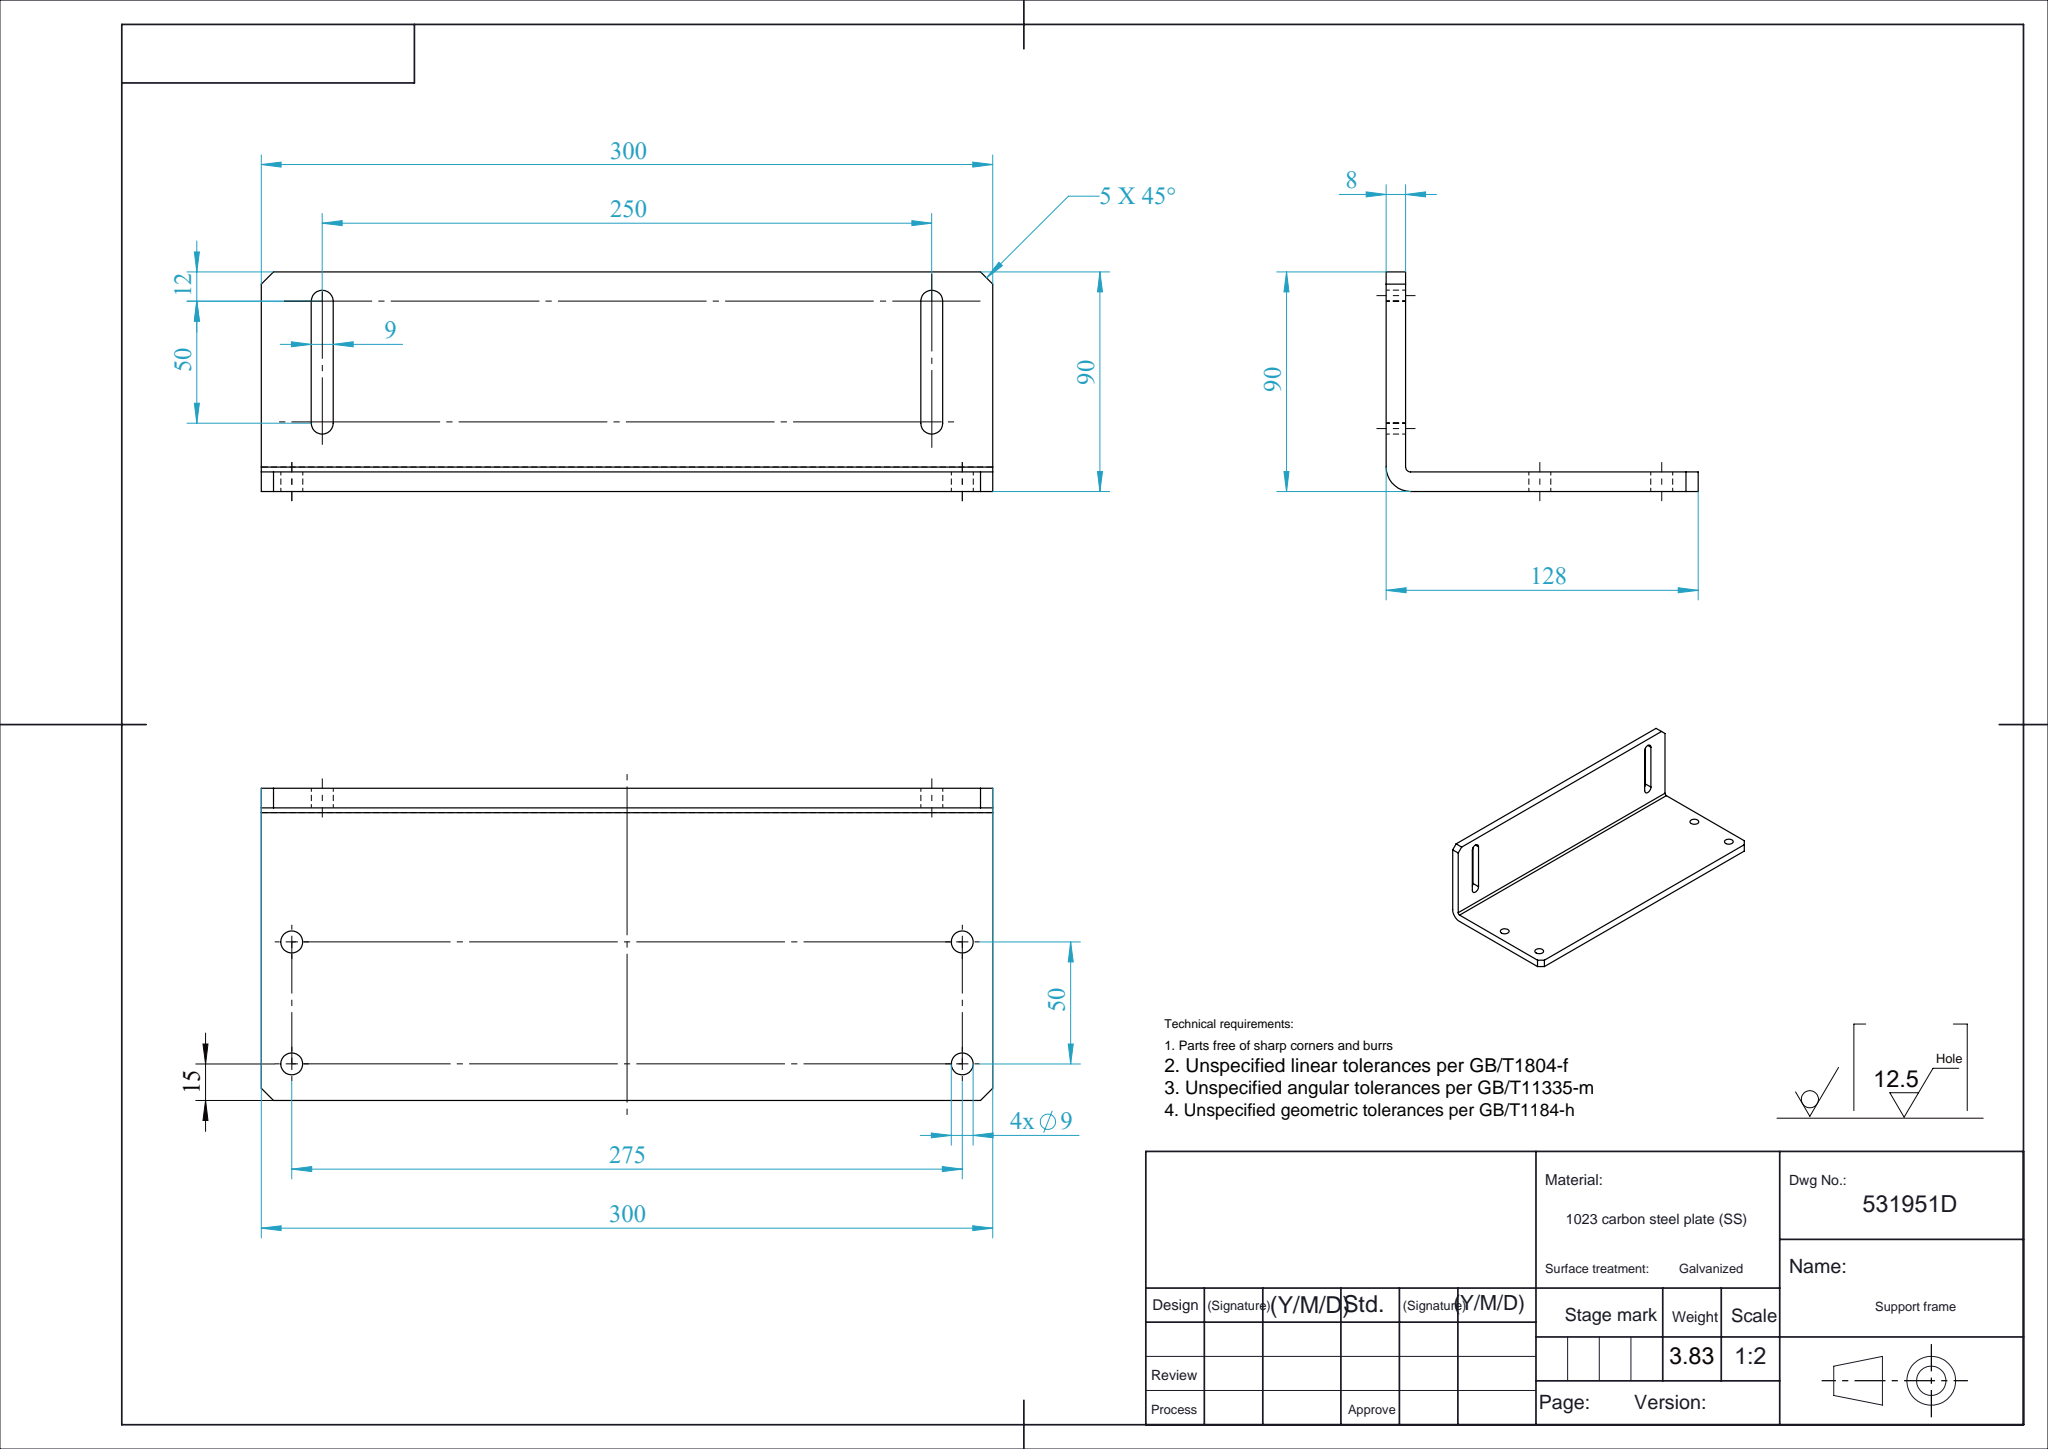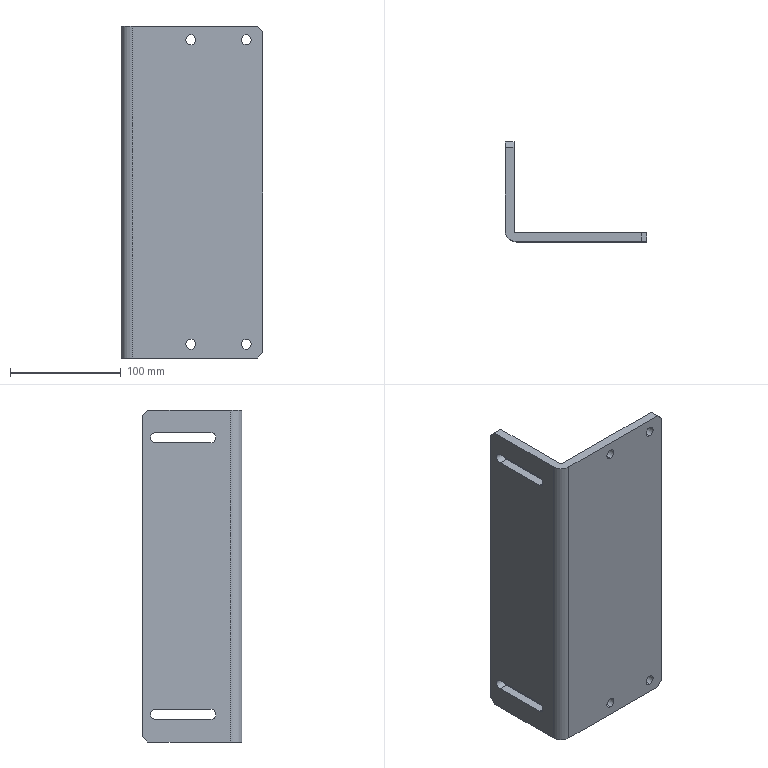Part | SolidWorks | features Fillet 2, ICE 2, Chamfer 1, Extrusion 1 | 1 solid | 30 faces | box 128 x 90 x 300 mm | volume 487166 mm3 | plane 16 | cylinder 14 | commonest cylinder face diameters 9 x12 4 x1 20 x1
STEP:
#1=CARTESIAN_POINT('',(113.,-90.,8.));
#2=VERTEX_POINT('',#1);
#3=CARTESIAN_POINT('',(113.,-90.,17.));
#4=VERTEX_POINT('',#3);
#5=CARTESIAN_POINT('',(113.,-90.,12.5));
#6=DIRECTION('',(0.,1.,0.));
#7=DIRECTION('',(0.,0.,1.));
#8=AXIS2_PLACEMENT_3D('',#5,#6,#7);
#9=CIRCLE('',#8,4.5);
#10=EDGE_CURVE('',#2,#4,#9,.T.);
#11=ORIENTED_EDGE('',*,*,#10,.F.);
#12=CARTESIAN_POINT('',(113.,-82.,8.));
#13=VERTEX_POINT('',#12);
#14=CARTESIAN_POINT('',(113.,-382.,8.));
#15=DIRECTION('',(0.,1.,0.));
#16=VECTOR('',#15,1000.);
#17=LINE('',#14,#16);
#18=EDGE_CURVE('',#2,#13,#17,.T.);
#19=ORIENTED_EDGE('',*,*,#18,.T.);
#20=CARTESIAN_POINT('',(113.,-82.,17.));
#21=VERTEX_POINT('',#20);
#22=CARTESIAN_POINT('',(113.,-82.,12.5));
#23=DIRECTION('',(0.,1.,0.));
#24=DIRECTION('',(0.,0.,1.));
#25=AXIS2_PLACEMENT_3D('',#22,#23,#24);
#26=CIRCLE('',#25,4.5);
#27=EDGE_CURVE('',#13,#21,#26,.T.);
#28=ORIENTED_EDGE('',*,*,#27,.T.);
#29=CARTESIAN_POINT('',(113.,-382.,17.));
#30=DIRECTION('',(0.,1.,0.));
#31=VECTOR('',#30,1000.);
#32=LINE('',#29,#31);
#33=EDGE_CURVE('',#4,#21,#32,.T.);
#34=ORIENTED_EDGE('',*,*,#33,.F.);
#35=EDGE_LOOP('',(#11,#19,#28,#34));
#36=FACE_OUTER_BOUND('',#35,.T.);
#37=CARTESIAN_POINT('',(113.,-382.,12.5));
#38=DIRECTION('',(0.,1.,0.));
#39=DIRECTION('',(0.,0.,1.));
#40=AXIS2_PLACEMENT_3D('',#37,#38,#39);
#41=CYLINDRICAL_SURFACE('',#40,4.5);
#42=ADVANCED_FACE('',(#36),#41,.F.);
#43=CARTESIAN_POINT('',(63.,-90.,283.));
#44=VERTEX_POINT('',#43);
#45=CARTESIAN_POINT('',(63.,-90.,292.));
#46=VERTEX_POINT('',#45);
#47=CARTESIAN_POINT('',(63.,-90.,287.5));
#48=DIRECTION('',(0.,1.,0.));
#49=DIRECTION('',(0.,0.,1.));
#50=AXIS2_PLACEMENT_3D('',#47,#48,#49);
#51=CIRCLE('',#50,4.5);
#52=EDGE_CURVE('',#44,#46,#51,.T.);
#53=ORIENTED_EDGE('',*,*,#52,.F.);
#54=CARTESIAN_POINT('',(63.,-82.,283.));
#55=VERTEX_POINT('',#54);
#56=CARTESIAN_POINT('',(63.,-382.,283.));
#57=DIRECTION('',(0.,1.,0.));
#58=VECTOR('',#57,1000.);
#59=LINE('',#56,#58);
#60=EDGE_CURVE('',#44,#55,#59,.T.);
#61=ORIENTED_EDGE('',*,*,#60,.T.);
#62=CARTESIAN_POINT('',(63.,-82.,292.));
#63=VERTEX_POINT('',#62);
#64=CARTESIAN_POINT('',(63.,-82.,287.5));
#65=DIRECTION('',(0.,1.,0.));
#66=DIRECTION('',(0.,0.,1.));
#67=AXIS2_PLACEMENT_3D('',#64,#65,#66);
#68=CIRCLE('',#67,4.5);
#69=EDGE_CURVE('',#55,#63,#68,.T.);
#70=ORIENTED_EDGE('',*,*,#69,.T.);
#71=CARTESIAN_POINT('',(63.,-382.,292.));
#72=DIRECTION('',(0.,1.,0.));
#73=VECTOR('',#72,1000.);
#74=LINE('',#71,#73);
#75=EDGE_CURVE('',#46,#63,#74,.T.);
#76=ORIENTED_EDGE('',*,*,#75,.F.);
#77=EDGE_LOOP('',(#53,#61,#70,#76));
#78=FACE_OUTER_BOUND('',#77,.T.);
#79=CARTESIAN_POINT('',(63.,-382.,287.5));
#80=DIRECTION('',(0.,1.,0.));
#81=DIRECTION('',(0.,0.,1.));
#82=AXIS2_PLACEMENT_3D('',#79,#80,#81);
#83=CYLINDRICAL_SURFACE('',#82,4.5);
#84=ADVANCED_FACE('',(#78),#83,.F.);
#85=CARTESIAN_POINT('',(113.,-90.,283.));
#86=VERTEX_POINT('',#85);
#87=CARTESIAN_POINT('',(113.,-90.,292.));
#88=VERTEX_POINT('',#87);
#89=CARTESIAN_POINT('',(113.,-90.,287.5));
#90=DIRECTION('',(0.,1.,0.));
#91=DIRECTION('',(0.,0.,1.));
#92=AXIS2_PLACEMENT_3D('',#89,#90,#91);
#93=CIRCLE('',#92,4.5);
#94=EDGE_CURVE('',#86,#88,#93,.T.);
#95=ORIENTED_EDGE('',*,*,#94,.F.);
#96=CARTESIAN_POINT('',(113.,-82.,283.));
#97=VERTEX_POINT('',#96);
#98=CARTESIAN_POINT('',(113.,-382.,283.));
#99=DIRECTION('',(0.,1.,0.));
#100=VECTOR('',#99,1000.);
#101=LINE('',#98,#100);
#102=EDGE_CURVE('',#86,#97,#101,.T.);
#103=ORIENTED_EDGE('',*,*,#102,.T.);
#104=CARTESIAN_POINT('',(113.,-82.,292.));
#105=VERTEX_POINT('',#104);
#106=CARTESIAN_POINT('',(113.,-82.,287.5));
#107=DIRECTION('',(0.,1.,0.));
#108=DIRECTION('',(0.,0.,1.));
#109=AXIS2_PLACEMENT_3D('',#106,#107,#108);
#110=CIRCLE('',#109,4.5);
#111=EDGE_CURVE('',#97,#105,#110,.T.);
#112=ORIENTED_EDGE('',*,*,#111,.T.);
#113=CARTESIAN_POINT('',(113.,-382.,292.));
#114=DIRECTION('',(0.,1.,0.));
#115=VECTOR('',#114,1000.);
#116=LINE('',#113,#115);
#117=EDGE_CURVE('',#88,#105,#116,.T.);
#118=ORIENTED_EDGE('',*,*,#117,.F.);
#119=EDGE_LOOP('',(#95,#103,#112,#118));
#120=FACE_OUTER_BOUND('',#119,.T.);
#121=CARTESIAN_POINT('',(113.,-382.,287.5));
#122=DIRECTION('',(0.,1.,0.));
#123=DIRECTION('',(0.,0.,1.));
#124=AXIS2_PLACEMENT_3D('',#121,#122,#123);
#125=CYLINDRICAL_SURFACE('',#124,4.5);
#126=ADVANCED_FACE('',(#120),#125,.F.);
#127=CARTESIAN_POINT('',(63.,-90.,8.));
#128=VERTEX_POINT('',#127);
#129=CARTESIAN_POINT('',(63.,-90.,17.));
#130=VERTEX_POINT('',#129);
#131=CARTESIAN_POINT('',(63.,-90.,12.5));
#132=DIRECTION('',(0.,1.,0.));
#133=DIRECTION('',(0.,0.,1.));
#134=AXIS2_PLACEMENT_3D('',#131,#132,#133);
#135=CIRCLE('',#134,4.5);
#136=EDGE_CURVE('',#128,#130,#135,.T.);
#137=ORIENTED_EDGE('',*,*,#136,.F.);
#138=CARTESIAN_POINT('',(63.,-82.,8.));
#139=VERTEX_POINT('',#138);
#140=CARTESIAN_POINT('',(63.,-382.,8.));
#141=DIRECTION('',(0.,1.,0.));
#142=VECTOR('',#141,1000.);
#143=LINE('',#140,#142);
#144=EDGE_CURVE('',#128,#139,#143,.T.);
#145=ORIENTED_EDGE('',*,*,#144,.T.);
#146=CARTESIAN_POINT('',(63.,-82.,17.));
#147=VERTEX_POINT('',#146);
#148=CARTESIAN_POINT('',(63.,-82.,12.5));
#149=DIRECTION('',(0.,1.,0.));
#150=DIRECTION('',(0.,0.,1.));
#151=AXIS2_PLACEMENT_3D('',#148,#149,#150);
#152=CIRCLE('',#151,4.5);
#153=EDGE_CURVE('',#139,#147,#152,.T.);
#154=ORIENTED_EDGE('',*,*,#153,.T.);
#155=CARTESIAN_POINT('',(63.,-382.,17.));
#156=DIRECTION('',(0.,1.,0.));
#157=VECTOR('',#156,1000.);
#158=LINE('',#155,#157);
#159=EDGE_CURVE('',#130,#147,#158,.T.);
#160=ORIENTED_EDGE('',*,*,#159,.F.);
#161=EDGE_LOOP('',(#137,#145,#154,#160));
#162=FACE_OUTER_BOUND('',#161,.T.);
#163=CARTESIAN_POINT('',(63.,-382.,12.5));
#164=DIRECTION('',(0.,1.,0.));
#165=DIRECTION('',(0.,0.,1.));
#166=AXIS2_PLACEMENT_3D('',#163,#164,#165);
#167=CYLINDRICAL_SURFACE('',#166,4.5);
#168=ADVANCED_FACE('',(#162),#167,.F.);
#169=CARTESIAN_POINT('',(113.,-82.,12.5));
#170=DIRECTION('',(0.,1.,0.));
#171=DIRECTION('',(0.,0.,1.));
#172=AXIS2_PLACEMENT_3D('',#169,#170,#171);
#173=CIRCLE('',#172,4.5);
#174=EDGE_CURVE('',#21,#13,#173,.T.);
#175=ORIENTED_EDGE('',*,*,#174,.F.);
#176=ORIENTED_EDGE('',*,*,#27,.F.);
#177=EDGE_LOOP('',(#175,#176));
#178=FACE_BOUND('',#177,.T.);
#179=CARTESIAN_POINT('',(63.,-82.,287.5));
#180=DIRECTION('',(0.,1.,0.));
#181=DIRECTION('',(0.,0.,1.));
#182=AXIS2_PLACEMENT_3D('',#179,#180,#181);
#183=CIRCLE('',#182,4.5);
#184=EDGE_CURVE('',#63,#55,#183,.T.);
#185=ORIENTED_EDGE('',*,*,#184,.F.);
#186=ORIENTED_EDGE('',*,*,#69,.F.);
#187=EDGE_LOOP('',(#185,#186));
#188=FACE_BOUND('',#187,.T.);
#189=CARTESIAN_POINT('',(113.,-82.,287.5));
#190=DIRECTION('',(0.,1.,0.));
#191=DIRECTION('',(0.,0.,1.));
#192=AXIS2_PLACEMENT_3D('',#189,#190,#191);
#193=CIRCLE('',#192,4.5);
#194=EDGE_CURVE('',#105,#97,#193,.T.);
#195=ORIENTED_EDGE('',*,*,#194,.F.);
#196=ORIENTED_EDGE('',*,*,#111,.F.);
#197=EDGE_LOOP('',(#195,#196));
#198=FACE_BOUND('',#197,.T.);
#199=CARTESIAN_POINT('',(63.,-82.,12.5));
#200=DIRECTION('',(0.,1.,0.));
#201=DIRECTION('',(0.,0.,1.));
#202=AXIS2_PLACEMENT_3D('',#199,#200,#201);
#203=CIRCLE('',#202,4.5);
#204=EDGE_CURVE('',#147,#139,#203,.T.);
#205=ORIENTED_EDGE('',*,*,#204,.F.);
#206=ORIENTED_EDGE('',*,*,#153,.F.);
#207=EDGE_LOOP('',(#205,#206));
#208=FACE_BOUND('',#207,.T.);
#209=CARTESIAN_POINT('',(10.,-82.,0.));
#210=VERTEX_POINT('',#209);
#211=CARTESIAN_POINT('',(123.,-82.,0.));
#212=VERTEX_POINT('',#211);
#213=CARTESIAN_POINT('',(8.,-82.,0.));
#214=DIRECTION('',(1.,0.,0.));
#215=VECTOR('',#214,1000.);
#216=LINE('',#213,#215);
#217=EDGE_CURVE('',#210,#212,#216,.T.);
#218=ORIENTED_EDGE('',*,*,#217,.F.);
#219=CARTESIAN_POINT('',(10.,-82.,300.));
#220=VERTEX_POINT('',#219);
#221=CARTESIAN_POINT('',(10.,-82.,300.));
#222=DIRECTION('',(0.,0.,1.));
#223=VECTOR('',#222,1000.);
#224=LINE('',#221,#223);
#225=EDGE_CURVE('',#210,#220,#224,.T.);
#226=ORIENTED_EDGE('',*,*,#225,.T.);
#227=CARTESIAN_POINT('',(123.,-82.,300.));
#228=VERTEX_POINT('',#227);
#229=CARTESIAN_POINT('',(8.,-82.,300.));
#230=DIRECTION('',(1.,0.,0.));
#231=VECTOR('',#230,1000.);
#232=LINE('',#229,#231);
#233=EDGE_CURVE('',#220,#228,#232,.T.);
#234=ORIENTED_EDGE('',*,*,#233,.T.);
#235=CARTESIAN_POINT('',(128.,-82.,295.));
#236=VERTEX_POINT('',#235);
#237=CARTESIAN_POINT('',(65.5,-82.,357.5));
#238=DIRECTION('',(0.7071,0.,-0.7071));
#239=VECTOR('',#238,1000.);
#240=LINE('',#237,#239);
#241=EDGE_CURVE('',#228,#236,#240,.T.);
#242=ORIENTED_EDGE('',*,*,#241,.T.);
#243=CARTESIAN_POINT('',(128.,-82.,5.));
#244=VERTEX_POINT('',#243);
#245=CARTESIAN_POINT('',(128.,-82.,300.));
#246=DIRECTION('',(0.,0.,-1.));
#247=VECTOR('',#246,1000.);
#248=LINE('',#245,#247);
#249=EDGE_CURVE('',#236,#244,#248,.T.);
#250=ORIENTED_EDGE('',*,*,#249,.T.);
#251=CARTESIAN_POINT('',(215.5,-82.,92.5));
#252=DIRECTION('',(-0.7071,0.,-0.7071));
#253=VECTOR('',#252,1000.);
#254=LINE('',#251,#253);
#255=EDGE_CURVE('',#244,#212,#254,.T.);
#256=ORIENTED_EDGE('',*,*,#255,.T.);
#257=EDGE_LOOP('',(#218,#226,#234,#242,#250,#256));
#258=FACE_OUTER_BOUND('',#257,.T.);
#259=CARTESIAN_POINT('',(8.,-82.,300.));
#260=DIRECTION('',(0.,1.,0.));
#261=DIRECTION('',(0.,0.,1.));
#262=AXIS2_PLACEMENT_3D('',#259,#260,#261);
#263=PLANE('',#262);
#264=ADVANCED_FACE('',(#178,#188,#198,#208,#258),#263,.T.);
#265=CARTESIAN_POINT('',(8.,-12.,270.5));
#266=VERTEX_POINT('',#265);
#267=CARTESIAN_POINT('',(8.,-12.,279.5));
#268=VERTEX_POINT('',#267);
#269=CARTESIAN_POINT('',(8.,-12.,275.));
#270=DIRECTION('',(1.,0.,0.));
#271=DIRECTION('',(0.,0.,-1.));
#272=AXIS2_PLACEMENT_3D('',#269,#270,#271);
#273=CIRCLE('',#272,4.5);
#274=EDGE_CURVE('',#266,#268,#273,.T.);
#275=ORIENTED_EDGE('',*,*,#274,.F.);
#276=CARTESIAN_POINT('',(8.,-62.,270.5));
#277=VERTEX_POINT('',#276);
#278=CARTESIAN_POINT('',(8.,-12.,270.5));
#279=DIRECTION('',(0.,1.,0.));
#280=VECTOR('',#279,1000.);
#281=LINE('',#278,#280);
#282=EDGE_CURVE('',#277,#266,#281,.T.);
#283=ORIENTED_EDGE('',*,*,#282,.F.);
#284=CARTESIAN_POINT('',(8.,-62.,279.5));
#285=VERTEX_POINT('',#284);
#286=CARTESIAN_POINT('',(8.,-62.,275.));
#287=DIRECTION('',(1.,0.,0.));
#288=DIRECTION('',(0.,0.,-1.));
#289=AXIS2_PLACEMENT_3D('',#286,#287,#288);
#290=CIRCLE('',#289,4.5);
#291=EDGE_CURVE('',#285,#277,#290,.T.);
#292=ORIENTED_EDGE('',*,*,#291,.F.);
#293=CARTESIAN_POINT('',(8.,-12.,279.5));
#294=DIRECTION('',(0.,-1.,0.));
#295=VECTOR('',#294,1000.);
#296=LINE('',#293,#295);
#297=EDGE_CURVE('',#268,#285,#296,.T.);
#298=ORIENTED_EDGE('',*,*,#297,.F.);
#299=EDGE_LOOP('',(#275,#283,#292,#298));
#300=FACE_BOUND('',#299,.T.);
#301=CARTESIAN_POINT('',(8.,-12.,20.5));
#302=VERTEX_POINT('',#301);
#303=CARTESIAN_POINT('',(8.,-12.,29.5));
#304=VERTEX_POINT('',#303);
#305=CARTESIAN_POINT('',(8.,-12.,25.));
#306=DIRECTION('',(1.,0.,0.));
#307=DIRECTION('',(0.,0.,1.));
#308=AXIS2_PLACEMENT_3D('',#305,#306,#307);
#309=CIRCLE('',#308,4.5);
#310=EDGE_CURVE('',#302,#304,#309,.T.);
#311=ORIENTED_EDGE('',*,*,#310,.F.);
#312=CARTESIAN_POINT('',(8.,-62.,20.5));
#313=VERTEX_POINT('',#312);
#314=CARTESIAN_POINT('',(8.,-12.,20.5));
#315=DIRECTION('',(0.,1.,0.));
#316=VECTOR('',#315,1000.);
#317=LINE('',#314,#316);
#318=EDGE_CURVE('',#313,#302,#317,.T.);
#319=ORIENTED_EDGE('',*,*,#318,.F.);
#320=CARTESIAN_POINT('',(8.,-62.,29.5));
#321=VERTEX_POINT('',#320);
#322=CARTESIAN_POINT('',(8.,-62.,25.));
#323=DIRECTION('',(1.,0.,0.));
#324=DIRECTION('',(0.,0.,1.));
#325=AXIS2_PLACEMENT_3D('',#322,#323,#324);
#326=CIRCLE('',#325,4.5);
#327=EDGE_CURVE('',#321,#313,#326,.T.);
#328=ORIENTED_EDGE('',*,*,#327,.F.);
#329=CARTESIAN_POINT('',(8.,-12.,29.5));
#330=DIRECTION('',(0.,-1.,0.));
#331=VECTOR('',#330,1000.);
#332=LINE('',#329,#331);
#333=EDGE_CURVE('',#304,#321,#332,.T.);
#334=ORIENTED_EDGE('',*,*,#333,.F.);
#335=EDGE_LOOP('',(#311,#319,#328,#334));
#336=FACE_BOUND('',#335,.T.);
#337=CARTESIAN_POINT('',(8.,-5.,300.));
#338=VERTEX_POINT('',#337);
#339=CARTESIAN_POINT('',(8.,-80.,300.));
#340=VERTEX_POINT('',#339);
#341=CARTESIAN_POINT('',(8.,0.,300.));
#342=DIRECTION('',(0.,-1.,0.));
#343=VECTOR('',#342,1000.);
#344=LINE('',#341,#343);
#345=EDGE_CURVE('',#338,#340,#344,.T.);
#346=ORIENTED_EDGE('',*,*,#345,.T.);
#347=CARTESIAN_POINT('',(8.,-80.,0.));
#348=VERTEX_POINT('',#347);
#349=CARTESIAN_POINT('',(8.,-80.,0.));
#350=DIRECTION('',(0.,0.,-1.));
#351=VECTOR('',#350,1000.);
#352=LINE('',#349,#351);
#353=EDGE_CURVE('',#340,#348,#352,.T.);
#354=ORIENTED_EDGE('',*,*,#353,.T.);
#355=CARTESIAN_POINT('',(8.,-5.,0.));
#356=VERTEX_POINT('',#355);
#357=CARTESIAN_POINT('',(8.,0.,0.));
#358=DIRECTION('',(0.,-1.,0.));
#359=VECTOR('',#358,1000.);
#360=LINE('',#357,#359);
#361=EDGE_CURVE('',#356,#348,#360,.T.);
#362=ORIENTED_EDGE('',*,*,#361,.F.);
#363=CARTESIAN_POINT('',(8.,0.,5.));
#364=VERTEX_POINT('',#363);
#365=CARTESIAN_POINT('',(8.,147.5,152.5));
#366=DIRECTION('',(0.,0.7071,0.7071));
#367=VECTOR('',#366,1000.);
#368=LINE('',#365,#367);
#369=EDGE_CURVE('',#356,#364,#368,.T.);
#370=ORIENTED_EDGE('',*,*,#369,.T.);
#371=CARTESIAN_POINT('',(8.,0.,295.));
#372=VERTEX_POINT('',#371);
#373=CARTESIAN_POINT('',(8.,0.,300.));
#374=DIRECTION('',(0.,0.,-1.));
#375=VECTOR('',#374,1000.);
#376=LINE('',#373,#375);
#377=EDGE_CURVE('',#372,#364,#376,.T.);
#378=ORIENTED_EDGE('',*,*,#377,.F.);
#379=CARTESIAN_POINT('',(8.,-2.5,297.5));
#380=DIRECTION('',(0.,-0.7071,0.7071));
#381=VECTOR('',#380,1000.);
#382=LINE('',#379,#381);
#383=EDGE_CURVE('',#372,#338,#382,.T.);
#384=ORIENTED_EDGE('',*,*,#383,.T.);
#385=EDGE_LOOP('',(#346,#354,#362,#370,#378,#384));
#386=FACE_OUTER_BOUND('',#385,.T.);
#387=CARTESIAN_POINT('',(8.,0.,300.));
#388=DIRECTION('',(1.,0.,0.));
#389=DIRECTION('',(0.,0.,-1.));
#390=AXIS2_PLACEMENT_3D('',#387,#388,#389);
#391=PLANE('',#390);
#392=ADVANCED_FACE('',(#300,#336,#386),#391,.T.);
#393=ORIENTED_EDGE('',*,*,#377,.T.);
#394=CARTESIAN_POINT('',(0.,0.,5.));
#395=VERTEX_POINT('',#394);
#396=CARTESIAN_POINT('',(0.,0.,5.));
#397=DIRECTION('',(-1.,0.,0.));
#398=VECTOR('',#397,1000.);
#399=LINE('',#396,#398);
#400=EDGE_CURVE('',#364,#395,#399,.T.);
#401=ORIENTED_EDGE('',*,*,#400,.T.);
#402=CARTESIAN_POINT('',(0.,0.,295.));
#403=VERTEX_POINT('',#402);
#404=CARTESIAN_POINT('',(0.,0.,300.));
#405=DIRECTION('',(0.,0.,-1.));
#406=VECTOR('',#405,1000.);
#407=LINE('',#404,#406);
#408=EDGE_CURVE('',#403,#395,#407,.T.);
#409=ORIENTED_EDGE('',*,*,#408,.F.);
#410=CARTESIAN_POINT('',(8.,0.,295.));
#411=DIRECTION('',(1.,0.,0.));
#412=VECTOR('',#411,1000.);
#413=LINE('',#410,#412);
#414=EDGE_CURVE('',#403,#372,#413,.T.);
#415=ORIENTED_EDGE('',*,*,#414,.T.);
#416=EDGE_LOOP('',(#393,#401,#409,#415));
#417=FACE_OUTER_BOUND('',#416,.T.);
#418=CARTESIAN_POINT('',(8.,0.,300.));
#419=DIRECTION('',(0.,-1.,0.));
#420=DIRECTION('',(0.,0.,-1.));
#421=AXIS2_PLACEMENT_3D('',#418,#419,#420);
#422=PLANE('',#421);
#423=ADVANCED_FACE('',(#417),#422,.F.);
#424=CARTESIAN_POINT('',(0.,-62.,270.5));
#425=VERTEX_POINT('',#424);
#426=CARTESIAN_POINT('',(0.,-12.,270.5));
#427=VERTEX_POINT('',#426);
#428=CARTESIAN_POINT('',(0.,0.,270.5));
#429=DIRECTION('',(0.,1.,0.));
#430=VECTOR('',#429,1000.);
#431=LINE('',#428,#430);
#432=EDGE_CURVE('',#425,#427,#431,.T.);
#433=ORIENTED_EDGE('',*,*,#432,.T.);
#434=CARTESIAN_POINT('',(0.,-12.,279.5));
#435=VERTEX_POINT('',#434);
#436=CARTESIAN_POINT('',(0.,-12.,275.));
#437=DIRECTION('',(1.,0.,0.));
#438=DIRECTION('',(0.,0.,-1.));
#439=AXIS2_PLACEMENT_3D('',#436,#437,#438);
#440=CIRCLE('',#439,4.5);
#441=EDGE_CURVE('',#427,#435,#440,.T.);
#442=ORIENTED_EDGE('',*,*,#441,.T.);
#443=CARTESIAN_POINT('',(0.,-62.,279.5));
#444=VERTEX_POINT('',#443);
#445=CARTESIAN_POINT('',(0.,0.,279.5));
#446=DIRECTION('',(0.,-1.,0.));
#447=VECTOR('',#446,1000.);
#448=LINE('',#445,#447);
#449=EDGE_CURVE('',#435,#444,#448,.T.);
#450=ORIENTED_EDGE('',*,*,#449,.T.);
#451=CARTESIAN_POINT('',(0.,-62.,275.));
#452=DIRECTION('',(1.,0.,0.));
#453=DIRECTION('',(0.,0.,-1.));
#454=AXIS2_PLACEMENT_3D('',#451,#452,#453);
#455=CIRCLE('',#454,4.5);
#456=EDGE_CURVE('',#444,#425,#455,.T.);
#457=ORIENTED_EDGE('',*,*,#456,.T.);
#458=EDGE_LOOP('',(#433,#442,#450,#457));
#459=FACE_BOUND('',#458,.T.);
#460=CARTESIAN_POINT('',(0.,-62.,20.5));
#461=VERTEX_POINT('',#460);
#462=CARTESIAN_POINT('',(0.,-12.,20.5));
#463=VERTEX_POINT('',#462);
#464=CARTESIAN_POINT('',(0.,0.,20.5));
#465=DIRECTION('',(0.,1.,0.));
#466=VECTOR('',#465,1000.);
#467=LINE('',#464,#466);
#468=EDGE_CURVE('',#461,#463,#467,.T.);
#469=ORIENTED_EDGE('',*,*,#468,.T.);
#470=CARTESIAN_POINT('',(0.,-12.,29.5));
#471=VERTEX_POINT('',#470);
#472=CARTESIAN_POINT('',(0.,-12.,25.));
#473=DIRECTION('',(1.,0.,0.));
#474=DIRECTION('',(0.,0.,-1.));
#475=AXIS2_PLACEMENT_3D('',#472,#473,#474);
#476=CIRCLE('',#475,4.5);
#477=EDGE_CURVE('',#463,#471,#476,.T.);
#478=ORIENTED_EDGE('',*,*,#477,.T.);
#479=CARTESIAN_POINT('',(0.,-62.,29.5));
#480=VERTEX_POINT('',#479);
#481=CARTESIAN_POINT('',(0.,0.,29.5));
#482=DIRECTION('',(0.,-1.,0.));
#483=VECTOR('',#482,1000.);
#484=LINE('',#481,#483);
#485=EDGE_CURVE('',#471,#480,#484,.T.);
#486=ORIENTED_EDGE('',*,*,#485,.T.);
#487=CARTESIAN_POINT('',(0.,-62.,25.));
#488=DIRECTION('',(1.,0.,0.));
#489=DIRECTION('',(0.,0.,-1.));
#490=AXIS2_PLACEMENT_3D('',#487,#488,#489);
#491=CIRCLE('',#490,4.5);
#492=EDGE_CURVE('',#480,#461,#491,.T.);
#493=ORIENTED_EDGE('',*,*,#492,.T.);
#494=EDGE_LOOP('',(#469,#478,#486,#493));
#495=FACE_BOUND('',#494,.T.);
#496=CARTESIAN_POINT('',(0.,-5.,0.));
#497=VERTEX_POINT('',#496);
#498=CARTESIAN_POINT('',(0.,-80.,0.));
#499=VERTEX_POINT('',#498);
#500=CARTESIAN_POINT('',(0.,0.,0.));
#501=DIRECTION('',(0.,-1.,0.));
#502=VECTOR('',#501,1000.);
#503=LINE('',#500,#502);
#504=EDGE_CURVE('',#497,#499,#503,.T.);
#505=ORIENTED_EDGE('',*,*,#504,.T.);
#506=CARTESIAN_POINT('',(0.,-80.,300.));
#507=VERTEX_POINT('',#506);
#508=CARTESIAN_POINT('',(0.,-80.,300.));
#509=DIRECTION('',(0.,0.,1.));
#510=VECTOR('',#509,1000.);
#511=LINE('',#508,#510);
#512=EDGE_CURVE('',#499,#507,#511,.T.);
#513=ORIENTED_EDGE('',*,*,#512,.T.);
#514=CARTESIAN_POINT('',(0.,-5.,300.));
#515=VERTEX_POINT('',#514);
#516=CARTESIAN_POINT('',(0.,0.,300.));
#517=DIRECTION('',(0.,-1.,0.));
#518=VECTOR('',#517,1000.);
#519=LINE('',#516,#518);
#520=EDGE_CURVE('',#515,#507,#519,.T.);
#521=ORIENTED_EDGE('',*,*,#520,.F.);
#522=CARTESIAN_POINT('',(0.,-5.,300.));
#523=DIRECTION('',(0.,0.7071,-0.7071));
#524=VECTOR('',#523,1000.);
#525=LINE('',#522,#524);
#526=EDGE_CURVE('',#515,#403,#525,.T.);
#527=ORIENTED_EDGE('',*,*,#526,.T.);
#528=ORIENTED_EDGE('',*,*,#408,.T.);
#529=CARTESIAN_POINT('',(0.,0.,5.));
#530=DIRECTION('',(0.,-0.7071,-0.7071));
#531=VECTOR('',#530,1000.);
#532=LINE('',#529,#531);
#533=EDGE_CURVE('',#395,#497,#532,.T.);
#534=ORIENTED_EDGE('',*,*,#533,.T.);
#535=EDGE_LOOP('',(#505,#513,#521,#527,#528,#534));
#536=FACE_OUTER_BOUND('',#535,.T.);
#537=CARTESIAN_POINT('',(0.,0.,300.));
#538=DIRECTION('',(1.,0.,0.));
#539=DIRECTION('',(0.,0.,-1.));
#540=AXIS2_PLACEMENT_3D('',#537,#538,#539);
#541=PLANE('',#540);
#542=ADVANCED_FACE('',(#459,#495,#536),#541,.F.);
#543=CARTESIAN_POINT('',(113.,-90.,12.5));
#544=DIRECTION('',(0.,1.,0.));
#545=DIRECTION('',(0.,0.,1.));
#546=AXIS2_PLACEMENT_3D('',#543,#544,#545);
#547=CIRCLE('',#546,4.5);
#548=EDGE_CURVE('',#4,#2,#547,.T.);
#549=ORIENTED_EDGE('',*,*,#548,.T.);
#550=ORIENTED_EDGE('',*,*,#10,.T.);
#551=EDGE_LOOP('',(#549,#550));
#552=FACE_BOUND('',#551,.T.);
#553=CARTESIAN_POINT('',(63.,-90.,287.5));
#554=DIRECTION('',(0.,1.,0.));
#555=DIRECTION('',(0.,0.,1.));
#556=AXIS2_PLACEMENT_3D('',#553,#554,#555);
#557=CIRCLE('',#556,4.5);
#558=EDGE_CURVE('',#46,#44,#557,.T.);
#559=ORIENTED_EDGE('',*,*,#558,.T.);
#560=ORIENTED_EDGE('',*,*,#52,.T.);
#561=EDGE_LOOP('',(#559,#560));
#562=FACE_BOUND('',#561,.T.);
#563=CARTESIAN_POINT('',(113.,-90.,287.5));
#564=DIRECTION('',(0.,1.,0.));
#565=DIRECTION('',(0.,0.,1.));
#566=AXIS2_PLACEMENT_3D('',#563,#564,#565);
#567=CIRCLE('',#566,4.5);
#568=EDGE_CURVE('',#88,#86,#567,.T.);
#569=ORIENTED_EDGE('',*,*,#568,.T.);
#570=ORIENTED_EDGE('',*,*,#94,.T.);
#571=EDGE_LOOP('',(#569,#570));
#572=FACE_BOUND('',#571,.T.);
#573=CARTESIAN_POINT('',(63.,-90.,12.5));
#574=DIRECTION('',(0.,1.,0.));
#575=DIRECTION('',(0.,0.,1.));
#576=AXIS2_PLACEMENT_3D('',#573,#574,#575);
#577=CIRCLE('',#576,4.5);
#578=EDGE_CURVE('',#130,#128,#577,.T.);
#579=ORIENTED_EDGE('',*,*,#578,.T.);
#580=ORIENTED_EDGE('',*,*,#136,.T.);
#581=EDGE_LOOP('',(#579,#580));
#582=FACE_BOUND('',#581,.T.);
#583=CARTESIAN_POINT('',(10.,-90.,300.));
#584=VERTEX_POINT('',#583);
#585=CARTESIAN_POINT('',(123.,-90.,300.));
#586=VERTEX_POINT('',#585);
#587=CARTESIAN_POINT('',(0.,-90.,300.));
#588=DIRECTION('',(1.,0.,0.));
#589=VECTOR('',#588,1000.);
#590=LINE('',#587,#589);
#591=EDGE_CURVE('',#584,#586,#590,.T.);
#592=ORIENTED_EDGE('',*,*,#591,.F.);
#593=CARTESIAN_POINT('',(10.,-90.,0.));
#594=VERTEX_POINT('',#593);
#595=CARTESIAN_POINT('',(10.,-90.,300.));
#596=DIRECTION('',(0.,0.,-1.));
#597=VECTOR('',#596,1000.);
#598=LINE('',#595,#597);
#599=EDGE_CURVE('',#584,#594,#598,.T.);
#600=ORIENTED_EDGE('',*,*,#599,.T.);
#601=CARTESIAN_POINT('',(123.,-90.,0.));
#602=VERTEX_POINT('',#601);
#603=CARTESIAN_POINT('',(0.,-90.,0.));
#604=DIRECTION('',(1.,0.,0.));
#605=VECTOR('',#604,1000.);
#606=LINE('',#603,#605);
#607=EDGE_CURVE('',#594,#602,#606,.T.);
#608=ORIENTED_EDGE('',*,*,#607,.T.);
#609=CARTESIAN_POINT('',(128.,-90.,5.));
#610=VERTEX_POINT('',#609);
#611=CARTESIAN_POINT('',(123.,-90.,0.));
#612=DIRECTION('',(0.7071,0.,0.7071));
#613=VECTOR('',#612,1000.);
#614=LINE('',#611,#613);
#615=EDGE_CURVE('',#602,#610,#614,.T.);
#616=ORIENTED_EDGE('',*,*,#615,.T.);
#617=CARTESIAN_POINT('',(128.,-90.,295.));
#618=VERTEX_POINT('',#617);
#619=CARTESIAN_POINT('',(128.,-90.,300.));
#620=DIRECTION('',(0.,0.,-1.));
#621=VECTOR('',#620,1000.);
#622=LINE('',#619,#621);
#623=EDGE_CURVE('',#618,#610,#622,.T.);
#624=ORIENTED_EDGE('',*,*,#623,.F.);
#625=CARTESIAN_POINT('',(128.,-90.,295.));
#626=DIRECTION('',(-0.7071,0.,0.7071));
#627=VECTOR('',#626,1000.);
#628=LINE('',#625,#627);
#629=EDGE_CURVE('',#618,#586,#628,.T.);
#630=ORIENTED_EDGE('',*,*,#629,.T.);
#631=EDGE_LOOP('',(#592,#600,#608,#616,#624,#630));
#632=FACE_OUTER_BOUND('',#631,.T.);
#633=CARTESIAN_POINT('',(0.,-90.,300.));
#634=DIRECTION('',(0.,1.,0.));
#635=DIRECTION('',(0.,0.,1.));
#636=AXIS2_PLACEMENT_3D('',#633,#634,#635);
#637=PLANE('',#636);
#638=ADVANCED_FACE('',(#552,#562,#572,#582,#632),#637,.F.);
#639=ORIENTED_EDGE('',*,*,#249,.F.);
#640=CARTESIAN_POINT('',(128.,-90.,295.));
#641=DIRECTION('',(0.,-1.,0.));
#642=VECTOR('',#641,1000.);
#643=LINE('',#640,#642);
#644=EDGE_CURVE('',#236,#618,#643,.T.);
#645=ORIENTED_EDGE('',*,*,#644,.T.);
#646=ORIENTED_EDGE('',*,*,#623,.T.);
#647=CARTESIAN_POINT('',(128.,-82.,5.));
#648=DIRECTION('',(0.,1.,0.));
#649=VECTOR('',#648,1000.);
#650=LINE('',#647,#649);
#651=EDGE_CURVE('',#610,#244,#650,.T.);
#652=ORIENTED_EDGE('',*,*,#651,.T.);
#653=EDGE_LOOP('',(#639,#645,#646,#652));
#654=FACE_OUTER_BOUND('',#653,.T.);
#655=CARTESIAN_POINT('',(128.,-82.,300.));
#656=DIRECTION('',(1.,0.,0.));
#657=DIRECTION('',(0.,0.,-1.));
#658=AXIS2_PLACEMENT_3D('',#655,#656,#657);
#659=PLANE('',#658);
#660=ADVANCED_FACE('',(#654),#659,.T.);
#661=ORIENTED_EDGE('',*,*,#520,.T.);
#662=CARTESIAN_POINT('',(10.,-80.,300.));
#663=DIRECTION('',(0.,0.,1.));
#664=DIRECTION('',(-1.,0.,0.));
#665=AXIS2_PLACEMENT_3D('',#662,#663,#664);
#666=CIRCLE('',#665,10.);
#667=EDGE_CURVE('',#507,#584,#666,.T.);
#668=ORIENTED_EDGE('',*,*,#667,.T.);
#669=ORIENTED_EDGE('',*,*,#591,.T.);
#670=CARTESIAN_POINT('',(123.,-82.,300.));
#671=DIRECTION('',(0.,1.,0.));
#672=VECTOR('',#671,1000.);
#673=LINE('',#670,#672);
#674=EDGE_CURVE('',#586,#228,#673,.T.);
#675=ORIENTED_EDGE('',*,*,#674,.T.);
#676=ORIENTED_EDGE('',*,*,#233,.F.);
#677=CARTESIAN_POINT('',(10.,-80.,300.));
#678=DIRECTION('',(0.,0.,-1.));
#679=DIRECTION('',(-1.,0.,0.));
#680=AXIS2_PLACEMENT_3D('',#677,#678,#679);
#681=CIRCLE('',#680,2.);
#682=EDGE_CURVE('',#220,#340,#681,.T.);
#683=ORIENTED_EDGE('',*,*,#682,.T.);
#684=ORIENTED_EDGE('',*,*,#345,.F.);
#685=CARTESIAN_POINT('',(0.,-5.,300.));
#686=DIRECTION('',(-1.,0.,0.));
#687=VECTOR('',#686,1000.);
#688=LINE('',#685,#687);
#689=EDGE_CURVE('',#338,#515,#688,.T.);
#690=ORIENTED_EDGE('',*,*,#689,.T.);
#691=EDGE_LOOP('',(#661,#668,#669,#675,#676,#683,#684,#690));
#692=FACE_OUTER_BOUND('',#691,.T.);
#693=CARTESIAN_POINT('',(0.,0.,300.));
#694=DIRECTION('',(0.,0.,-1.));
#695=DIRECTION('',(-1.,0.,0.));
#696=AXIS2_PLACEMENT_3D('',#693,#694,#695);
#697=PLANE('',#696);
#698=ADVANCED_FACE('',(#692),#697,.F.);
#699=ORIENTED_EDGE('',*,*,#607,.F.);
#700=CARTESIAN_POINT('',(10.,-80.,0.));
#701=DIRECTION('',(0.,0.,-1.));
#702=DIRECTION('',(-1.,0.,0.));
#703=AXIS2_PLACEMENT_3D('',#700,#701,#702);
#704=CIRCLE('',#703,10.);
#705=EDGE_CURVE('',#594,#499,#704,.T.);
#706=ORIENTED_EDGE('',*,*,#705,.T.);
#707=ORIENTED_EDGE('',*,*,#504,.F.);
#708=CARTESIAN_POINT('',(8.,-5.,0.));
#709=DIRECTION('',(1.,0.,0.));
#710=VECTOR('',#709,1000.);
#711=LINE('',#708,#710);
#712=EDGE_CURVE('',#497,#356,#711,.T.);
#713=ORIENTED_EDGE('',*,*,#712,.T.);
#714=ORIENTED_EDGE('',*,*,#361,.T.);
#715=CARTESIAN_POINT('',(10.,-80.,0.));
#716=DIRECTION('',(0.,0.,1.));
#717=DIRECTION('',(-1.,0.,0.));
#718=AXIS2_PLACEMENT_3D('',#715,#716,#717);
#719=CIRCLE('',#718,2.);
#720=EDGE_CURVE('',#348,#210,#719,.T.);
#721=ORIENTED_EDGE('',*,*,#720,.T.);
#722=ORIENTED_EDGE('',*,*,#217,.T.);
#723=CARTESIAN_POINT('',(123.,0.,0.));
#724=DIRECTION('',(0.,-1.,0.));
#725=VECTOR('',#724,1000.);
#726=LINE('',#723,#725);
#727=EDGE_CURVE('',#212,#602,#726,.T.);
#728=ORIENTED_EDGE('',*,*,#727,.T.);
#729=EDGE_LOOP('',(#699,#706,#707,#713,#714,#721,#722,#728));
#730=FACE_OUTER_BOUND('',#729,.T.);
#731=CARTESIAN_POINT('',(0.,0.,0.));
#732=DIRECTION('',(0.,0.,-1.));
#733=DIRECTION('',(-1.,0.,0.));
#734=AXIS2_PLACEMENT_3D('',#731,#732,#733);
#735=PLANE('',#734);
#736=ADVANCED_FACE('',(#730),#735,.T.);
#737=ORIENTED_EDGE('',*,*,#144,.F.);
#738=ORIENTED_EDGE('',*,*,#578,.F.);
#739=ORIENTED_EDGE('',*,*,#159,.T.);
#740=ORIENTED_EDGE('',*,*,#204,.T.);
#741=EDGE_LOOP('',(#737,#738,#739,#740));
#742=FACE_OUTER_BOUND('',#741,.T.);
#743=CARTESIAN_POINT('',(63.,-382.,12.5));
#744=DIRECTION('',(0.,1.,0.));
#745=DIRECTION('',(0.,0.,1.));
#746=AXIS2_PLACEMENT_3D('',#743,#744,#745);
#747=CYLINDRICAL_SURFACE('',#746,4.5);
#748=ADVANCED_FACE('',(#742),#747,.F.);
#749=ORIENTED_EDGE('',*,*,#102,.F.);
#750=ORIENTED_EDGE('',*,*,#568,.F.);
#751=ORIENTED_EDGE('',*,*,#117,.T.);
#752=ORIENTED_EDGE('',*,*,#194,.T.);
#753=EDGE_LOOP('',(#749,#750,#751,#752));
#754=FACE_OUTER_BOUND('',#753,.T.);
#755=CARTESIAN_POINT('',(113.,-382.,287.5));
#756=DIRECTION('',(0.,1.,0.));
#757=DIRECTION('',(0.,0.,1.));
#758=AXIS2_PLACEMENT_3D('',#755,#756,#757);
#759=CYLINDRICAL_SURFACE('',#758,4.5);
#760=ADVANCED_FACE('',(#754),#759,.F.);
#761=ORIENTED_EDGE('',*,*,#60,.F.);
#762=ORIENTED_EDGE('',*,*,#558,.F.);
#763=ORIENTED_EDGE('',*,*,#75,.T.);
#764=ORIENTED_EDGE('',*,*,#184,.T.);
#765=EDGE_LOOP('',(#761,#762,#763,#764));
#766=FACE_OUTER_BOUND('',#765,.T.);
#767=CARTESIAN_POINT('',(63.,-382.,287.5));
#768=DIRECTION('',(0.,1.,0.));
#769=DIRECTION('',(0.,0.,1.));
#770=AXIS2_PLACEMENT_3D('',#767,#768,#769);
#771=CYLINDRICAL_SURFACE('',#770,4.5);
#772=ADVANCED_FACE('',(#766),#771,.F.);
#773=ORIENTED_EDGE('',*,*,#18,.F.);
#774=ORIENTED_EDGE('',*,*,#548,.F.);
#775=ORIENTED_EDGE('',*,*,#33,.T.);
#776=ORIENTED_EDGE('',*,*,#174,.T.);
#777=EDGE_LOOP('',(#773,#774,#775,#776));
#778=FACE_OUTER_BOUND('',#777,.T.);
#779=CARTESIAN_POINT('',(113.,-382.,12.5));
#780=DIRECTION('',(0.,1.,0.));
#781=DIRECTION('',(0.,0.,1.));
#782=AXIS2_PLACEMENT_3D('',#779,#780,#781);
#783=CYLINDRICAL_SURFACE('',#782,4.5);
#784=ADVANCED_FACE('',(#778),#783,.F.);
#785=CARTESIAN_POINT('',(-292.,-12.,20.5));
#786=DIRECTION('',(1.,0.,0.));
#787=VECTOR('',#786,1000.);
#788=LINE('',#785,#787);
#789=EDGE_CURVE('',#463,#302,#788,.T.);
#790=ORIENTED_EDGE('',*,*,#789,.T.);
#791=ORIENTED_EDGE('',*,*,#310,.T.);
#792=CARTESIAN_POINT('',(-292.,-12.,29.5));
#793=DIRECTION('',(1.,0.,0.));
#794=VECTOR('',#793,1000.);
#795=LINE('',#792,#794);
#796=EDGE_CURVE('',#471,#304,#795,.T.);
#797=ORIENTED_EDGE('',*,*,#796,.F.);
#798=ORIENTED_EDGE('',*,*,#477,.F.);
#799=EDGE_LOOP('',(#790,#791,#797,#798));
#800=FACE_OUTER_BOUND('',#799,.T.);
#801=CARTESIAN_POINT('',(-292.,-12.,25.));
#802=DIRECTION('',(1.,0.,0.));
#803=DIRECTION('',(0.,0.,-1.));
#804=AXIS2_PLACEMENT_3D('',#801,#802,#803);
#805=CYLINDRICAL_SURFACE('',#804,4.5);
#806=ADVANCED_FACE('',(#800),#805,.F.);
#807=CARTESIAN_POINT('',(-292.,-62.,20.5));
#808=DIRECTION('',(1.,0.,0.));
#809=VECTOR('',#808,1000.);
#810=LINE('',#807,#809);
#811=EDGE_CURVE('',#461,#313,#810,.T.);
#812=ORIENTED_EDGE('',*,*,#811,.T.);
#813=ORIENTED_EDGE('',*,*,#318,.T.);
#814=ORIENTED_EDGE('',*,*,#789,.F.);
#815=ORIENTED_EDGE('',*,*,#468,.F.);
#816=EDGE_LOOP('',(#812,#813,#814,#815));
#817=FACE_OUTER_BOUND('',#816,.T.);
#818=CARTESIAN_POINT('',(-292.,-12.,20.5));
#819=DIRECTION('',(0.,0.,-1.));
#820=DIRECTION('',(-1.,0.,0.));
#821=AXIS2_PLACEMENT_3D('',#818,#819,#820);
#822=PLANE('',#821);
#823=ADVANCED_FACE('',(#817),#822,.F.);
#824=CARTESIAN_POINT('',(-292.,-62.,29.5));
#825=DIRECTION('',(1.,0.,0.));
#826=VECTOR('',#825,1000.);
#827=LINE('',#824,#826);
#828=EDGE_CURVE('',#480,#321,#827,.T.);
#829=ORIENTED_EDGE('',*,*,#828,.T.);
#830=ORIENTED_EDGE('',*,*,#327,.T.);
#831=ORIENTED_EDGE('',*,*,#811,.F.);
#832=ORIENTED_EDGE('',*,*,#492,.F.);
#833=EDGE_LOOP('',(#829,#830,#831,#832));
#834=FACE_OUTER_BOUND('',#833,.T.);
#835=CARTESIAN_POINT('',(-292.,-62.,25.));
#836=DIRECTION('',(1.,0.,0.));
#837=DIRECTION('',(0.,0.,-1.));
#838=AXIS2_PLACEMENT_3D('',#835,#836,#837);
#839=CYLINDRICAL_SURFACE('',#838,4.5);
#840=ADVANCED_FACE('',(#834),#839,.F.);
#841=ORIENTED_EDGE('',*,*,#796,.T.);
#842=ORIENTED_EDGE('',*,*,#333,.T.);
#843=ORIENTED_EDGE('',*,*,#828,.F.);
#844=ORIENTED_EDGE('',*,*,#485,.F.);
#845=EDGE_LOOP('',(#841,#842,#843,#844));
#846=FACE_OUTER_BOUND('',#845,.T.);
#847=CARTESIAN_POINT('',(-292.,-12.,29.5));
#848=DIRECTION('',(0.,0.,1.));
#849=DIRECTION('',(1.,0.,0.));
#850=AXIS2_PLACEMENT_3D('',#847,#848,#849);
#851=PLANE('',#850);
#852=ADVANCED_FACE('',(#846),#851,.F.);
#853=CARTESIAN_POINT('',(-292.,-12.,270.5));
#854=DIRECTION('',(1.,0.,0.));
#855=VECTOR('',#854,1000.);
#856=LINE('',#853,#855);
#857=EDGE_CURVE('',#427,#266,#856,.T.);
#858=ORIENTED_EDGE('',*,*,#857,.T.);
#859=ORIENTED_EDGE('',*,*,#274,.T.);
#860=CARTESIAN_POINT('',(-292.,-12.,279.5));
#861=DIRECTION('',(1.,0.,0.));
#862=VECTOR('',#861,1000.);
#863=LINE('',#860,#862);
#864=EDGE_CURVE('',#435,#268,#863,.T.);
#865=ORIENTED_EDGE('',*,*,#864,.F.);
#866=ORIENTED_EDGE('',*,*,#441,.F.);
#867=EDGE_LOOP('',(#858,#859,#865,#866));
#868=FACE_OUTER_BOUND('',#867,.T.);
#869=CARTESIAN_POINT('',(-292.,-12.,275.));
#870=DIRECTION('',(1.,0.,0.));
#871=DIRECTION('',(0.,0.,-1.));
#872=AXIS2_PLACEMENT_3D('',#869,#870,#871);
#873=CYLINDRICAL_SURFACE('',#872,4.5);
#874=ADVANCED_FACE('',(#868),#873,.F.);
#875=CARTESIAN_POINT('',(-292.,-62.,270.5));
#876=DIRECTION('',(1.,0.,0.));
#877=VECTOR('',#876,1000.);
#878=LINE('',#875,#877);
#879=EDGE_CURVE('',#425,#277,#878,.T.);
#880=ORIENTED_EDGE('',*,*,#879,.T.);
#881=ORIENTED_EDGE('',*,*,#282,.T.);
#882=ORIENTED_EDGE('',*,*,#857,.F.);
#883=ORIENTED_EDGE('',*,*,#432,.F.);
#884=EDGE_LOOP('',(#880,#881,#882,#883));
#885=FACE_OUTER_BOUND('',#884,.T.);
#886=CARTESIAN_POINT('',(-292.,-12.,270.5));
#887=DIRECTION('',(0.,0.,-1.));
#888=DIRECTION('',(-1.,0.,0.));
#889=AXIS2_PLACEMENT_3D('',#886,#887,#888);
#890=PLANE('',#889);
#891=ADVANCED_FACE('',(#885),#890,.F.);
#892=CARTESIAN_POINT('',(-292.,-62.,279.5));
#893=DIRECTION('',(1.,0.,0.));
#894=VECTOR('',#893,1000.);
#895=LINE('',#892,#894);
#896=EDGE_CURVE('',#444,#285,#895,.T.);
#897=ORIENTED_EDGE('',*,*,#896,.T.);
#898=ORIENTED_EDGE('',*,*,#291,.T.);
#899=ORIENTED_EDGE('',*,*,#879,.F.);
#900=ORIENTED_EDGE('',*,*,#456,.F.);
#901=EDGE_LOOP('',(#897,#898,#899,#900));
#902=FACE_OUTER_BOUND('',#901,.T.);
#903=CARTESIAN_POINT('',(-292.,-62.,275.));
#904=DIRECTION('',(1.,0.,0.));
#905=DIRECTION('',(0.,0.,-1.));
#906=AXIS2_PLACEMENT_3D('',#903,#904,#905);
#907=CYLINDRICAL_SURFACE('',#906,4.5);
#908=ADVANCED_FACE('',(#902),#907,.F.);
#909=ORIENTED_EDGE('',*,*,#864,.T.);
#910=ORIENTED_EDGE('',*,*,#297,.T.);
#911=ORIENTED_EDGE('',*,*,#896,.F.);
#912=ORIENTED_EDGE('',*,*,#449,.F.);
#913=EDGE_LOOP('',(#909,#910,#911,#912));
#914=FACE_OUTER_BOUND('',#913,.T.);
#915=CARTESIAN_POINT('',(-292.,-12.,279.5));
#916=DIRECTION('',(0.,0.,1.));
#917=DIRECTION('',(1.,0.,0.));
#918=AXIS2_PLACEMENT_3D('',#915,#916,#917);
#919=PLANE('',#918);
#920=ADVANCED_FACE('',(#914),#919,.F.);
#921=ORIENTED_EDGE('',*,*,#241,.F.);
#922=ORIENTED_EDGE('',*,*,#674,.F.);
#923=ORIENTED_EDGE('',*,*,#629,.F.);
#924=ORIENTED_EDGE('',*,*,#644,.F.);
#925=EDGE_LOOP('',(#921,#922,#923,#924));
#926=FACE_OUTER_BOUND('',#925,.T.);
#927=CARTESIAN_POINT('',(128.,-82.,295.));
#928=DIRECTION('',(0.7071,0.,0.7071));
#929=DIRECTION('',(0.,1.,0.));
#930=AXIS2_PLACEMENT_3D('',#927,#928,#929);
#931=PLANE('',#930);
#932=ADVANCED_FACE('',(#926),#931,.T.);
#933=ORIENTED_EDGE('',*,*,#255,.F.);
#934=ORIENTED_EDGE('',*,*,#651,.F.);
#935=ORIENTED_EDGE('',*,*,#615,.F.);
#936=ORIENTED_EDGE('',*,*,#727,.F.);
#937=EDGE_LOOP('',(#933,#934,#935,#936));
#938=FACE_OUTER_BOUND('',#937,.T.);
#939=CARTESIAN_POINT('',(123.,0.,0.));
#940=DIRECTION('',(-0.7071,0.,0.7071));
#941=DIRECTION('',(0.,-1.,0.));
#942=AXIS2_PLACEMENT_3D('',#939,#940,#941);
#943=PLANE('',#942);
#944=ADVANCED_FACE('',(#938),#943,.F.);
#945=ORIENTED_EDGE('',*,*,#369,.F.);
#946=ORIENTED_EDGE('',*,*,#712,.F.);
#947=ORIENTED_EDGE('',*,*,#533,.F.);
#948=ORIENTED_EDGE('',*,*,#400,.F.);
#949=EDGE_LOOP('',(#945,#946,#947,#948));
#950=FACE_OUTER_BOUND('',#949,.T.);
#951=CARTESIAN_POINT('',(8.,0.,5.));
#952=DIRECTION('',(0.,0.7071,-0.7071));
#953=DIRECTION('',(1.,0.,0.));
#954=AXIS2_PLACEMENT_3D('',#951,#952,#953);
#955=PLANE('',#954);
#956=ADVANCED_FACE('',(#950),#955,.T.);
#957=ORIENTED_EDGE('',*,*,#383,.F.);
#958=ORIENTED_EDGE('',*,*,#414,.F.);
#959=ORIENTED_EDGE('',*,*,#526,.F.);
#960=ORIENTED_EDGE('',*,*,#689,.F.);
#961=EDGE_LOOP('',(#957,#958,#959,#960));
#962=FACE_OUTER_BOUND('',#961,.T.);
#963=CARTESIAN_POINT('',(0.,-5.,300.));
#964=DIRECTION('',(0.,-0.7071,-0.7071));
#965=DIRECTION('',(-1.,0.,0.));
#966=AXIS2_PLACEMENT_3D('',#963,#964,#965);
#967=PLANE('',#966);
#968=ADVANCED_FACE('',(#962),#967,.F.);
#969=ORIENTED_EDGE('',*,*,#682,.F.);
#970=ORIENTED_EDGE('',*,*,#225,.F.);
#971=ORIENTED_EDGE('',*,*,#720,.F.);
#972=ORIENTED_EDGE('',*,*,#353,.F.);
#973=EDGE_LOOP('',(#969,#970,#971,#972));
#974=FACE_OUTER_BOUND('',#973,.T.);
#975=CARTESIAN_POINT('',(10.,-80.,300.));
#976=DIRECTION('',(0.,0.,1.));
#977=DIRECTION('',(1.,0.,0.));
#978=AXIS2_PLACEMENT_3D('',#975,#976,#977);
#979=CYLINDRICAL_SURFACE('',#978,2.);
#980=ADVANCED_FACE('',(#974),#979,.F.);
#981=ORIENTED_EDGE('',*,*,#667,.F.);
#982=ORIENTED_EDGE('',*,*,#512,.F.);
#983=ORIENTED_EDGE('',*,*,#705,.F.);
#984=ORIENTED_EDGE('',*,*,#599,.F.);
#985=EDGE_LOOP('',(#981,#982,#983,#984));
#986=FACE_OUTER_BOUND('',#985,.T.);
#987=CARTESIAN_POINT('',(10.,-80.,300.));
#988=DIRECTION('',(0.,0.,-1.));
#989=DIRECTION('',(-1.,0.,0.));
#990=AXIS2_PLACEMENT_3D('',#987,#988,#989);
#991=CYLINDRICAL_SURFACE('',#990,10.);
#992=ADVANCED_FACE('',(#986),#991,.T.);
#993=CLOSED_SHELL('',(#42,#84,#126,#168,#264,#392,#423,#542,#638,#660,#698,#736,#748,#760,#772,#784,#806,#823,#840,#852,#874,#891,#908,#920,#932,#944,#956,#968,#980,#992));
#994=MANIFOLD_SOLID_BREP('',#993);
#995=CARTESIAN_POINT('',(0.,0.,0.));
#996=DIRECTION('',(0.,0.,1.));
#997=DIRECTION('',(1.,0.,0.));
#998=AXIS2_PLACEMENT_3D('',#995,#996,#997);
#999=(LENGTH_UNIT()NAMED_UNIT(*)SI_UNIT(.MILLI.,.METRE.));
#1000=UNCERTAINTY_MEASURE_WITH_UNIT(LENGTH_MEASURE(0.00001),#999,'','');
#1001=(NAMED_UNIT(*)PLANE_ANGLE_UNIT()SI_UNIT($,.RADIAN.));
#1002=(NAMED_UNIT(*)SI_UNIT($,.STERADIAN.)SOLID_ANGLE_UNIT());
#1003=(GEOMETRIC_REPRESENTATION_CONTEXT(3)GLOBAL_UNCERTAINTY_ASSIGNED_CONTEXT((#1000))GLOBAL_UNIT_ASSIGNED_CONTEXT((#999,#1001,#1002))REPRESENTATION_CONTEXT('',''));
#1004=ADVANCED_BREP_SHAPE_REPRESENTATION('',(#994,#998),#1003);